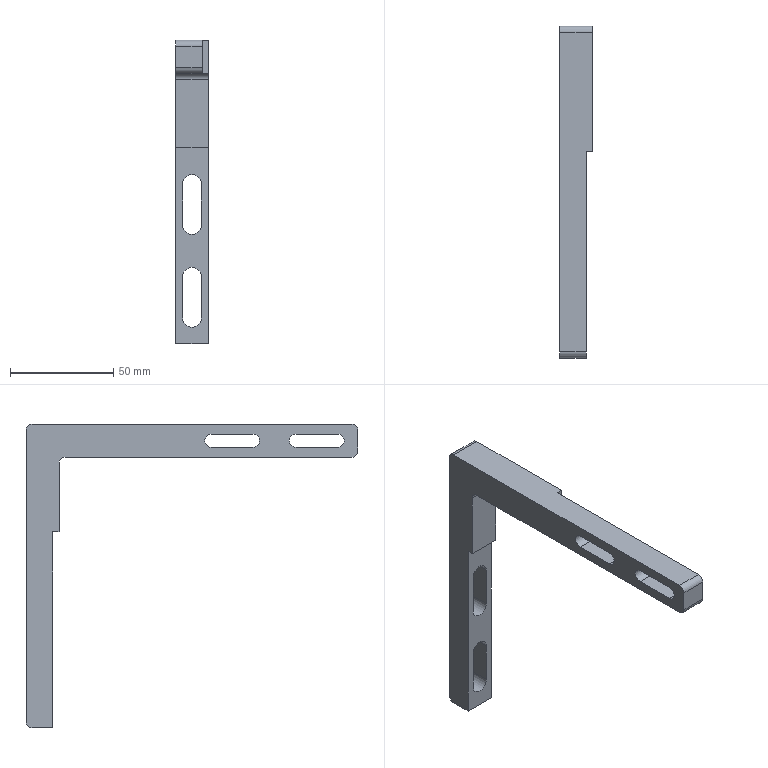Part | STEP file | SN10_019_003_SUPORTE | 1 solid | 33 faces | box 16 x 161 x 147.15 mm | volume 54772 mm3 | plane 20 | cylinder 13 | commonest cylinder face diameters 6 x5 6.5 x4 9 x4